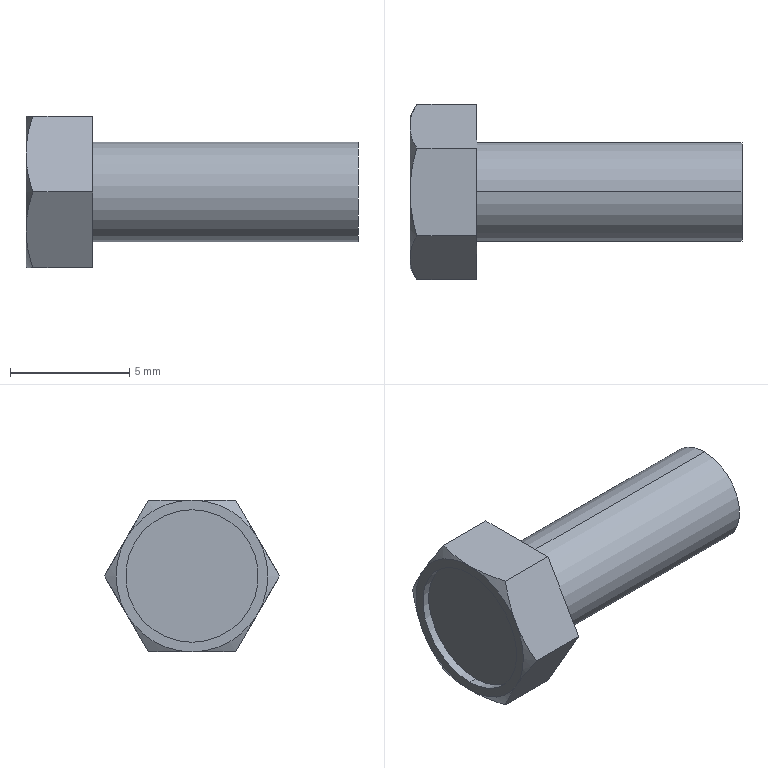Part | SolidWorks | features BaseBody 1 | 1 solid | 20 faces | box 13.907 x 7.332 x 6.35 mm | volume 240.264 mm3 | plane 10 | cone 6 | cylinder 4 | commonest cylinder face diameters 4.166 x2 5.556 x2
STEP:
#1=CARTESIAN_POINT('',(0.3493,0.,2.778));
#2=VERTEX_POINT('',#1);
#3=CARTESIAN_POINT('',(0.3493,0.,-2.778));
#4=VERTEX_POINT('',#3);
#5=CARTESIAN_POINT('',(0.3493,0.,0.));
#6=DIRECTION('',(1.,0.,0.));
#7=DIRECTION('',(0.,0.,1.));
#8=AXIS2_PLACEMENT_3D('',#5,#6,#7);
#9=CIRCLE('',#8,2.778);
#10=EDGE_CURVE('',#2,#4,#9,.T.);
#11=ORIENTED_EDGE('',*,*,#10,.T.);
#12=CARTESIAN_POINT('',(0.,0.,-2.778));
#13=VERTEX_POINT('',#12);
#14=CARTESIAN_POINT('',(0.3493,0.,-2.778));
#15=DIRECTION('',(-1.,0.,0.));
#16=VECTOR('',#15,1000.);
#17=LINE('',#14,#16);
#18=EDGE_CURVE('',#4,#13,#17,.T.);
#19=ORIENTED_EDGE('',*,*,#18,.T.);
#20=CARTESIAN_POINT('',(0.,0.,2.778));
#21=VERTEX_POINT('',#20);
#22=CARTESIAN_POINT('',(0.,0.,0.));
#23=DIRECTION('',(-1.,0.,0.));
#24=DIRECTION('',(0.,0.,1.));
#25=AXIS2_PLACEMENT_3D('',#22,#23,#24);
#26=CIRCLE('',#25,2.778);
#27=EDGE_CURVE('',#13,#21,#26,.T.);
#28=ORIENTED_EDGE('',*,*,#27,.T.);
#29=CARTESIAN_POINT('',(0.3493,0.,2.778));
#30=DIRECTION('',(-1.,0.,0.));
#31=VECTOR('',#30,1000.);
#32=LINE('',#29,#31);
#33=EDGE_CURVE('',#2,#21,#32,.T.);
#34=ORIENTED_EDGE('',*,*,#33,.F.);
#35=EDGE_LOOP('',(#11,#19,#28,#34));
#36=FACE_OUTER_BOUND('',#35,.T.);
#37=CARTESIAN_POINT('',(0.3493,0.,0.));
#38=DIRECTION('',(-1.,0.,0.));
#39=DIRECTION('',(0.,0.,1.));
#40=AXIS2_PLACEMENT_3D('',#37,#38,#39);
#41=CYLINDRICAL_SURFACE('',#40,2.778);
#42=ADVANCED_FACE('',(#36),#41,.F.);
#43=CARTESIAN_POINT('',(13.907,0.,-2.083));
#44=VERTEX_POINT('',#43);
#45=CARTESIAN_POINT('',(13.907,0.,2.083));
#46=VERTEX_POINT('',#45);
#47=CARTESIAN_POINT('',(13.907,0.,0.));
#48=DIRECTION('',(1.,0.,0.));
#49=DIRECTION('',(0.,0.,1.));
#50=AXIS2_PLACEMENT_3D('',#47,#48,#49);
#51=CIRCLE('',#50,2.083);
#52=EDGE_CURVE('',#44,#46,#51,.T.);
#53=ORIENTED_EDGE('',*,*,#52,.F.);
#54=CARTESIAN_POINT('',(2.794,0.,-2.083));
#55=VERTEX_POINT('',#54);
#56=CARTESIAN_POINT('',(13.907,0.,-2.083));
#57=DIRECTION('',(-1.,0.,0.));
#58=VECTOR('',#57,1000.);
#59=LINE('',#56,#58);
#60=EDGE_CURVE('',#44,#55,#59,.T.);
#61=ORIENTED_EDGE('',*,*,#60,.T.);
#62=CARTESIAN_POINT('',(2.794,0.,2.083));
#63=VERTEX_POINT('',#62);
#64=CARTESIAN_POINT('',(2.794,0.,0.));
#65=DIRECTION('',(1.,0.,0.));
#66=DIRECTION('',(0.,0.,1.));
#67=AXIS2_PLACEMENT_3D('',#64,#65,#66);
#68=CIRCLE('',#67,2.083);
#69=EDGE_CURVE('',#55,#63,#68,.T.);
#70=ORIENTED_EDGE('',*,*,#69,.T.);
#71=CARTESIAN_POINT('',(13.907,0.,2.083));
#72=DIRECTION('',(-1.,0.,0.));
#73=VECTOR('',#72,1000.);
#74=LINE('',#71,#73);
#75=EDGE_CURVE('',#46,#63,#74,.T.);
#76=ORIENTED_EDGE('',*,*,#75,.F.);
#77=EDGE_LOOP('',(#53,#61,#70,#76));
#78=FACE_OUTER_BOUND('',#77,.T.);
#79=CARTESIAN_POINT('',(13.907,0.,0.));
#80=DIRECTION('',(-1.,0.,0.));
#81=DIRECTION('',(0.,0.,1.));
#82=AXIS2_PLACEMENT_3D('',#79,#80,#81);
#83=CYLINDRICAL_SURFACE('',#82,2.083);
#84=ADVANCED_FACE('',(#78),#83,.T.);
#85=ORIENTED_EDGE('',*,*,#18,.F.);
#86=CARTESIAN_POINT('',(0.3493,0.,0.));
#87=DIRECTION('',(1.,0.,0.));
#88=DIRECTION('',(0.,0.,1.));
#89=AXIS2_PLACEMENT_3D('',#86,#87,#88);
#90=CIRCLE('',#89,2.778);
#91=EDGE_CURVE('',#4,#2,#90,.T.);
#92=ORIENTED_EDGE('',*,*,#91,.T.);
#93=ORIENTED_EDGE('',*,*,#33,.T.);
#94=CARTESIAN_POINT('',(0.,0.,0.));
#95=DIRECTION('',(-1.,0.,0.));
#96=DIRECTION('',(0.,0.,1.));
#97=AXIS2_PLACEMENT_3D('',#94,#95,#96);
#98=CIRCLE('',#97,2.778);
#99=EDGE_CURVE('',#21,#13,#98,.T.);
#100=ORIENTED_EDGE('',*,*,#99,.T.);
#101=EDGE_LOOP('',(#85,#92,#93,#100));
#102=FACE_OUTER_BOUND('',#101,.T.);
#103=CARTESIAN_POINT('',(0.3493,0.,0.));
#104=DIRECTION('',(-1.,0.,0.));
#105=DIRECTION('',(0.,0.,1.));
#106=AXIS2_PLACEMENT_3D('',#103,#104,#105);
#107=CYLINDRICAL_SURFACE('',#106,2.778);
#108=ADVANCED_FACE('',(#102),#107,.F.);
#109=ORIENTED_EDGE('',*,*,#99,.F.);
#110=ORIENTED_EDGE('',*,*,#27,.F.);
#111=EDGE_LOOP('',(#109,#110));
#112=FACE_BOUND('',#111,.T.);
#113=CARTESIAN_POINT('',(0.000000003,-2.75,-1.588));
#114=VERTEX_POINT('',#113);
#115=CARTESIAN_POINT('',(0.000000006,-2.75,1.588));
#116=VERTEX_POINT('',#115);
#117=CARTESIAN_POINT('',(0.000000006,0.,0.));
#118=DIRECTION('',(-1.,0.,0.));
#119=DIRECTION('',(0.,0.,-1.));
#120=AXIS2_PLACEMENT_3D('',#117,#118,#119);
#121=CIRCLE('',#120,3.175);
#122=EDGE_CURVE('',#114,#116,#121,.T.);
#123=ORIENTED_EDGE('',*,*,#122,.T.);
#124=CARTESIAN_POINT('',(0.,-0.000000001,3.175));
#125=VERTEX_POINT('',#124);
#126=CARTESIAN_POINT('',(0.,0.,0.));
#127=DIRECTION('',(-1.,0.,0.));
#128=DIRECTION('',(0.,0.,-1.));
#129=AXIS2_PLACEMENT_3D('',#126,#127,#128);
#130=CIRCLE('',#129,3.175);
#131=EDGE_CURVE('',#116,#125,#130,.T.);
#132=ORIENTED_EDGE('',*,*,#131,.T.);
#133=CARTESIAN_POINT('',(0.000000003,2.75,1.588));
#134=VERTEX_POINT('',#133);
#135=CARTESIAN_POINT('',(0.,0.,0.));
#136=DIRECTION('',(-1.,0.,0.));
#137=DIRECTION('',(0.,0.,-1.));
#138=AXIS2_PLACEMENT_3D('',#135,#136,#137);
#139=CIRCLE('',#138,3.175);
#140=EDGE_CURVE('',#125,#134,#139,.T.);
#141=ORIENTED_EDGE('',*,*,#140,.T.);
#142=CARTESIAN_POINT('',(0.000000006,2.75,-1.588));
#143=VERTEX_POINT('',#142);
#144=CARTESIAN_POINT('',(0.000000006,0.,0.));
#145=DIRECTION('',(-1.,0.,0.));
#146=DIRECTION('',(0.,0.,-1.));
#147=AXIS2_PLACEMENT_3D('',#144,#145,#146);
#148=CIRCLE('',#147,3.175);
#149=EDGE_CURVE('',#134,#143,#148,.T.);
#150=ORIENTED_EDGE('',*,*,#149,.T.);
#151=CARTESIAN_POINT('',(0.000000003,0.,-3.175));
#152=VERTEX_POINT('',#151);
#153=CARTESIAN_POINT('',(0.000000006,0.,0.));
#154=DIRECTION('',(-1.,0.,0.));
#155=DIRECTION('',(0.,0.,-1.));
#156=AXIS2_PLACEMENT_3D('',#153,#154,#155);
#157=CIRCLE('',#156,3.175);
#158=EDGE_CURVE('',#143,#152,#157,.T.);
#159=ORIENTED_EDGE('',*,*,#158,.T.);
#160=CARTESIAN_POINT('',(0.,0.,0.));
#161=DIRECTION('',(-1.,0.,0.));
#162=DIRECTION('',(0.,0.,-1.));
#163=AXIS2_PLACEMENT_3D('',#160,#161,#162);
#164=CIRCLE('',#163,3.175);
#165=EDGE_CURVE('',#152,#114,#164,.T.);
#166=ORIENTED_EDGE('',*,*,#165,.T.);
#167=EDGE_LOOP('',(#123,#132,#141,#150,#159,#166));
#168=FACE_OUTER_BOUND('',#167,.T.);
#169=CARTESIAN_POINT('',(0.,-3.213,-3.213));
#170=DIRECTION('',(-1.,0.,0.));
#171=DIRECTION('',(0.,0.,1.));
#172=AXIS2_PLACEMENT_3D('',#169,#170,#171);
#173=PLANE('',#172);
#174=ADVANCED_FACE('',(#112,#168),#173,.T.);
#175=ORIENTED_EDGE('',*,*,#10,.F.);
#176=ORIENTED_EDGE('',*,*,#91,.F.);
#177=EDGE_LOOP('',(#175,#176));
#178=FACE_OUTER_BOUND('',#177,.T.);
#179=CARTESIAN_POINT('',(0.3493,-2.811,2.811));
#180=DIRECTION('',(1.,0.,0.));
#181=DIRECTION('',(0.,0.,-1.));
#182=AXIS2_PLACEMENT_3D('',#179,#180,#181);
#183=PLANE('',#182);
#184=ADVANCED_FACE('',(#178),#183,.F.);
#185=CARTESIAN_POINT('',(0.2836,-1.833,3.175));
#186=VERTEX_POINT('',#185);
#187=CARTESIAN_POINT('',(0.2836,-1.833,3.175));
#188=CARTESIAN_POINT('',(0.1107,-2.133,2.656));
#189=CARTESIAN_POINT('',(0.000000006,-2.437,2.129));
#190=CARTESIAN_POINT('',(0.000000006,-2.75,1.588));
#191=B_SPLINE_CURVE_WITH_KNOTS('',3,(#187,#188,#189,#190),.UNSPECIFIED.,.F.,.F.,(4,4),(0.,0.001855),.UNSPECIFIED.);
#192=EDGE_CURVE('',#186,#116,#191,.T.);
#193=ORIENTED_EDGE('',*,*,#192,.F.);
#194=CARTESIAN_POINT('',(0.,-0.000000001,3.175));
#195=CARTESIAN_POINT('',(0.,-0.6257,3.175));
#196=CARTESIAN_POINT('',(0.1107,-1.234,3.175));
#197=CARTESIAN_POINT('',(0.2836,-1.833,3.175));
#198=B_SPLINE_CURVE_WITH_KNOTS('',3,(#194,#195,#196,#197),.UNSPECIFIED.,.F.,.F.,(4,4),(0.,0.001855),.UNSPECIFIED.);
#199=EDGE_CURVE('',#125,#186,#198,.T.);
#200=ORIENTED_EDGE('',*,*,#199,.F.);
#201=ORIENTED_EDGE('',*,*,#131,.F.);
#202=EDGE_LOOP('',(#193,#200,#201));
#203=FACE_OUTER_BOUND('',#202,.T.);
#204=CARTESIAN_POINT('',(0.,0.,0.));
#205=DIRECTION('',(1.,0.,0.));
#206=DIRECTION('',(0.,0.,-1.));
#207=AXIS2_PLACEMENT_3D('',#204,#205,#206);
#208=CONICAL_SURFACE('',#207,3.175,1.047);
#209=ADVANCED_FACE('',(#203),#208,.T.);
#210=CARTESIAN_POINT('',(0.2836,-3.666,0.));
#211=VERTEX_POINT('',#210);
#212=CARTESIAN_POINT('',(0.2836,-3.666,0.));
#213=CARTESIAN_POINT('',(0.1107,-3.367,-0.5187));
#214=CARTESIAN_POINT('',(0.000000006,-3.062,-1.046));
#215=CARTESIAN_POINT('',(0.000000003,-2.75,-1.588));
#216=B_SPLINE_CURVE_WITH_KNOTS('',3,(#212,#213,#214,#215),.UNSPECIFIED.,.F.,.F.,(4,4),(0.,0.001855),.UNSPECIFIED.);
#217=EDGE_CURVE('',#211,#114,#216,.T.);
#218=ORIENTED_EDGE('',*,*,#217,.F.);
#219=CARTESIAN_POINT('',(0.000000006,-2.75,1.588));
#220=CARTESIAN_POINT('',(0.000000006,-3.062,1.046));
#221=CARTESIAN_POINT('',(0.1107,-3.367,0.5187));
#222=CARTESIAN_POINT('',(0.2836,-3.666,0.));
#223=B_SPLINE_CURVE_WITH_KNOTS('',3,(#219,#220,#221,#222),.UNSPECIFIED.,.F.,.F.,(4,4),(0.,0.001855),.UNSPECIFIED.);
#224=EDGE_CURVE('',#116,#211,#223,.T.);
#225=ORIENTED_EDGE('',*,*,#224,.F.);
#226=ORIENTED_EDGE('',*,*,#122,.F.);
#227=EDGE_LOOP('',(#218,#225,#226));
#228=FACE_OUTER_BOUND('',#227,.T.);
#229=CARTESIAN_POINT('',(0.000000006,0.,0.));
#230=DIRECTION('',(1.,0.,0.));
#231=DIRECTION('',(0.,0.,-1.));
#232=AXIS2_PLACEMENT_3D('',#229,#230,#231);
#233=CONICAL_SURFACE('',#232,3.175,1.047);
#234=ADVANCED_FACE('',(#228),#233,.T.);
#235=CARTESIAN_POINT('',(0.2836,-1.833,-3.175));
#236=VERTEX_POINT('',#235);
#237=CARTESIAN_POINT('',(0.000000003,-2.75,-1.588));
#238=CARTESIAN_POINT('',(0.000000006,-2.437,-2.129));
#239=CARTESIAN_POINT('',(0.1107,-2.133,-2.656));
#240=CARTESIAN_POINT('',(0.2836,-1.833,-3.175));
#241=B_SPLINE_CURVE_WITH_KNOTS('',3,(#237,#238,#239,#240),.UNSPECIFIED.,.F.,.F.,(4,4),(0.,0.001855),.UNSPECIFIED.);
#242=EDGE_CURVE('',#114,#236,#241,.T.);
#243=ORIENTED_EDGE('',*,*,#242,.F.);
#244=ORIENTED_EDGE('',*,*,#165,.F.);
#245=CARTESIAN_POINT('',(0.2836,-1.833,-3.175));
#246=CARTESIAN_POINT('',(0.1107,-1.234,-3.175));
#247=CARTESIAN_POINT('',(0.,-0.6257,-3.175));
#248=CARTESIAN_POINT('',(0.000000003,0.,-3.175));
#249=B_SPLINE_CURVE_WITH_KNOTS('',3,(#245,#246,#247,#248),.UNSPECIFIED.,.F.,.F.,(4,4),(0.,0.001855),.UNSPECIFIED.);
#250=EDGE_CURVE('',#236,#152,#249,.T.);
#251=ORIENTED_EDGE('',*,*,#250,.F.);
#252=EDGE_LOOP('',(#243,#244,#251));
#253=FACE_OUTER_BOUND('',#252,.T.);
#254=CARTESIAN_POINT('',(0.,0.,0.));
#255=DIRECTION('',(1.,0.,0.));
#256=DIRECTION('',(0.,0.,-1.));
#257=AXIS2_PLACEMENT_3D('',#254,#255,#256);
#258=CONICAL_SURFACE('',#257,3.175,1.047);
#259=ADVANCED_FACE('',(#253),#258,.T.);
#260=CARTESIAN_POINT('',(0.2836,1.833,-3.175));
#261=VERTEX_POINT('',#260);
#262=CARTESIAN_POINT('',(0.000000003,0.,-3.175));
#263=CARTESIAN_POINT('',(0.,0.6257,-3.175));
#264=CARTESIAN_POINT('',(0.1107,1.234,-3.175));
#265=CARTESIAN_POINT('',(0.2836,1.833,-3.175));
#266=B_SPLINE_CURVE_WITH_KNOTS('',3,(#262,#263,#264,#265),.UNSPECIFIED.,.F.,.F.,(4,4),(0.,0.001855),.UNSPECIFIED.);
#267=EDGE_CURVE('',#152,#261,#266,.T.);
#268=ORIENTED_EDGE('',*,*,#267,.F.);
#269=ORIENTED_EDGE('',*,*,#158,.F.);
#270=CARTESIAN_POINT('',(0.2836,1.833,-3.175));
#271=CARTESIAN_POINT('',(0.1107,2.133,-2.656));
#272=CARTESIAN_POINT('',(0.000000006,2.437,-2.129));
#273=CARTESIAN_POINT('',(0.000000006,2.75,-1.588));
#274=B_SPLINE_CURVE_WITH_KNOTS('',3,(#270,#271,#272,#273),.UNSPECIFIED.,.F.,.F.,(4,4),(0.,0.001855),.UNSPECIFIED.);
#275=EDGE_CURVE('',#261,#143,#274,.T.);
#276=ORIENTED_EDGE('',*,*,#275,.F.);
#277=EDGE_LOOP('',(#268,#269,#276));
#278=FACE_OUTER_BOUND('',#277,.T.);
#279=CARTESIAN_POINT('',(0.,0.,0.));
#280=DIRECTION('',(1.,0.,0.));
#281=DIRECTION('',(0.,0.,-1.));
#282=AXIS2_PLACEMENT_3D('',#279,#280,#281);
#283=CONICAL_SURFACE('',#282,3.175,1.047);
#284=ADVANCED_FACE('',(#278),#283,.T.);
#285=CARTESIAN_POINT('',(0.2836,3.666,0.));
#286=VERTEX_POINT('',#285);
#287=CARTESIAN_POINT('',(0.000000006,2.75,-1.588));
#288=CARTESIAN_POINT('',(0.000000006,3.062,-1.046));
#289=CARTESIAN_POINT('',(0.1107,3.367,-0.5187));
#290=CARTESIAN_POINT('',(0.2836,3.666,0.));
#291=B_SPLINE_CURVE_WITH_KNOTS('',3,(#287,#288,#289,#290),.UNSPECIFIED.,.F.,.F.,(4,4),(0.,0.001855),.UNSPECIFIED.);
#292=EDGE_CURVE('',#143,#286,#291,.T.);
#293=ORIENTED_EDGE('',*,*,#292,.F.);
#294=ORIENTED_EDGE('',*,*,#149,.F.);
#295=CARTESIAN_POINT('',(0.2836,3.666,0.));
#296=CARTESIAN_POINT('',(0.1107,3.367,0.5187));
#297=CARTESIAN_POINT('',(0.000000006,3.062,1.046));
#298=CARTESIAN_POINT('',(0.000000003,2.75,1.588));
#299=B_SPLINE_CURVE_WITH_KNOTS('',3,(#295,#296,#297,#298),.UNSPECIFIED.,.F.,.F.,(4,4),(0.,0.001855),.UNSPECIFIED.);
#300=EDGE_CURVE('',#286,#134,#299,.T.);
#301=ORIENTED_EDGE('',*,*,#300,.F.);
#302=EDGE_LOOP('',(#293,#294,#301));
#303=FACE_OUTER_BOUND('',#302,.T.);
#304=CARTESIAN_POINT('',(0.000000006,0.,0.));
#305=DIRECTION('',(1.,0.,0.));
#306=DIRECTION('',(0.,0.,-1.));
#307=AXIS2_PLACEMENT_3D('',#304,#305,#306);
#308=CONICAL_SURFACE('',#307,3.175,1.047);
#309=ADVANCED_FACE('',(#303),#308,.T.);
#310=CARTESIAN_POINT('',(0.2836,1.833,3.175));
#311=VERTEX_POINT('',#310);
#312=CARTESIAN_POINT('',(0.2836,1.833,3.175));
#313=CARTESIAN_POINT('',(0.1107,1.234,3.175));
#314=CARTESIAN_POINT('',(0.,0.6257,3.175));
#315=CARTESIAN_POINT('',(0.,-0.000000001,3.175));
#316=B_SPLINE_CURVE_WITH_KNOTS('',3,(#312,#313,#314,#315),.UNSPECIFIED.,.F.,.F.,(4,4),(0.,0.001855),.UNSPECIFIED.);
#317=EDGE_CURVE('',#311,#125,#316,.T.);
#318=ORIENTED_EDGE('',*,*,#317,.F.);
#319=CARTESIAN_POINT('',(0.000000003,2.75,1.588));
#320=CARTESIAN_POINT('',(0.000000006,2.437,2.129));
#321=CARTESIAN_POINT('',(0.1107,2.133,2.656));
#322=CARTESIAN_POINT('',(0.2836,1.833,3.175));
#323=B_SPLINE_CURVE_WITH_KNOTS('',3,(#319,#320,#321,#322),.UNSPECIFIED.,.F.,.F.,(4,4),(0.,0.001855),.UNSPECIFIED.);
#324=EDGE_CURVE('',#134,#311,#323,.T.);
#325=ORIENTED_EDGE('',*,*,#324,.F.);
#326=ORIENTED_EDGE('',*,*,#140,.F.);
#327=EDGE_LOOP('',(#318,#325,#326));
#328=FACE_OUTER_BOUND('',#327,.T.);
#329=CARTESIAN_POINT('',(0.,0.,0.));
#330=DIRECTION('',(1.,0.,0.));
#331=DIRECTION('',(0.,0.,-1.));
#332=AXIS2_PLACEMENT_3D('',#329,#330,#331);
#333=CONICAL_SURFACE('',#332,3.175,1.047);
#334=ADVANCED_FACE('',(#328),#333,.T.);
#335=ORIENTED_EDGE('',*,*,#192,.T.);
#336=ORIENTED_EDGE('',*,*,#224,.T.);
#337=CARTESIAN_POINT('',(2.794,-3.666,0.));
#338=VERTEX_POINT('',#337);
#339=CARTESIAN_POINT('',(1.389,-3.666,0.));
#340=DIRECTION('',(1.,0.,0.));
#341=VECTOR('',#340,1000.);
#342=LINE('',#339,#341);
#343=EDGE_CURVE('',#211,#338,#342,.T.);
#344=ORIENTED_EDGE('',*,*,#343,.T.);
#345=CARTESIAN_POINT('',(2.794,-1.833,3.175));
#346=VERTEX_POINT('',#345);
#347=CARTESIAN_POINT('',(2.794,-2.75,1.587));
#348=DIRECTION('',(0.,0.5,0.866));
#349=VECTOR('',#348,1000.);
#350=LINE('',#347,#349);
#351=EDGE_CURVE('',#338,#346,#350,.T.);
#352=ORIENTED_EDGE('',*,*,#351,.T.);
#353=CARTESIAN_POINT('',(1.389,-1.833,3.175));
#354=DIRECTION('',(-1.,0.,0.));
#355=VECTOR('',#354,1000.);
#356=LINE('',#353,#355);
#357=EDGE_CURVE('',#346,#186,#356,.T.);
#358=ORIENTED_EDGE('',*,*,#357,.T.);
#359=EDGE_LOOP('',(#335,#336,#344,#352,#358));
#360=FACE_OUTER_BOUND('',#359,.T.);
#361=CARTESIAN_POINT('',(-0.01676,-1.833,3.175));
#362=DIRECTION('',(0.,-0.866,0.5));
#363=DIRECTION('',(0.,-0.5,-0.866));
#364=AXIS2_PLACEMENT_3D('',#361,#362,#363);
#365=PLANE('',#364);
#366=ADVANCED_FACE('',(#360),#365,.T.);
#367=ORIENTED_EDGE('',*,*,#317,.T.);
#368=ORIENTED_EDGE('',*,*,#199,.T.);
#369=ORIENTED_EDGE('',*,*,#357,.F.);
#370=CARTESIAN_POINT('',(2.794,1.833,3.175));
#371=VERTEX_POINT('',#370);
#372=CARTESIAN_POINT('',(2.794,0.,3.175));
#373=DIRECTION('',(0.,1.,0.));
#374=VECTOR('',#373,1000.);
#375=LINE('',#372,#374);
#376=EDGE_CURVE('',#346,#371,#375,.T.);
#377=ORIENTED_EDGE('',*,*,#376,.T.);
#378=CARTESIAN_POINT('',(1.389,1.833,3.175));
#379=DIRECTION('',(-1.,0.,0.));
#380=VECTOR('',#379,1000.);
#381=LINE('',#378,#380);
#382=EDGE_CURVE('',#371,#311,#381,.T.);
#383=ORIENTED_EDGE('',*,*,#382,.T.);
#384=EDGE_LOOP('',(#367,#368,#369,#377,#383));
#385=FACE_OUTER_BOUND('',#384,.T.);
#386=CARTESIAN_POINT('',(-0.01676,1.833,3.175));
#387=DIRECTION('',(0.,0.,1.));
#388=DIRECTION('',(0.,-1.,0.));
#389=AXIS2_PLACEMENT_3D('',#386,#387,#388);
#390=PLANE('',#389);
#391=ADVANCED_FACE('',(#385),#390,.T.);
#392=ORIENTED_EDGE('',*,*,#217,.T.);
#393=ORIENTED_EDGE('',*,*,#242,.T.);
#394=CARTESIAN_POINT('',(2.794,-1.833,-3.175));
#395=VERTEX_POINT('',#394);
#396=CARTESIAN_POINT('',(1.389,-1.833,-3.175));
#397=DIRECTION('',(1.,0.,0.));
#398=VECTOR('',#397,1000.);
#399=LINE('',#396,#398);
#400=EDGE_CURVE('',#236,#395,#399,.T.);
#401=ORIENTED_EDGE('',*,*,#400,.T.);
#402=CARTESIAN_POINT('',(2.794,-2.75,-1.587));
#403=DIRECTION('',(0.,-0.5,0.866));
#404=VECTOR('',#403,1000.);
#405=LINE('',#402,#404);
#406=EDGE_CURVE('',#395,#338,#405,.T.);
#407=ORIENTED_EDGE('',*,*,#406,.T.);
#408=ORIENTED_EDGE('',*,*,#343,.F.);
#409=EDGE_LOOP('',(#392,#393,#401,#407,#408));
#410=FACE_OUTER_BOUND('',#409,.T.);
#411=CARTESIAN_POINT('',(-0.01676,-3.666,0.));
#412=DIRECTION('',(0.,-0.866,-0.5));
#413=DIRECTION('',(0.,0.5,-0.866));
#414=AXIS2_PLACEMENT_3D('',#411,#412,#413);
#415=PLANE('',#414);
#416=ADVANCED_FACE('',(#410),#415,.T.);
#417=ORIENTED_EDGE('',*,*,#250,.T.);
#418=ORIENTED_EDGE('',*,*,#267,.T.);
#419=CARTESIAN_POINT('',(2.794,1.833,-3.175));
#420=VERTEX_POINT('',#419);
#421=CARTESIAN_POINT('',(1.389,1.833,-3.175));
#422=DIRECTION('',(1.,0.,0.));
#423=VECTOR('',#422,1000.);
#424=LINE('',#421,#423);
#425=EDGE_CURVE('',#261,#420,#424,.T.);
#426=ORIENTED_EDGE('',*,*,#425,.T.);
#427=CARTESIAN_POINT('',(2.794,0.,-3.175));
#428=DIRECTION('',(0.,-1.,0.));
#429=VECTOR('',#428,1000.);
#430=LINE('',#427,#429);
#431=EDGE_CURVE('',#420,#395,#430,.T.);
#432=ORIENTED_EDGE('',*,*,#431,.T.);
#433=ORIENTED_EDGE('',*,*,#400,.F.);
#434=EDGE_LOOP('',(#417,#418,#426,#432,#433));
#435=FACE_OUTER_BOUND('',#434,.T.);
#436=CARTESIAN_POINT('',(-0.01676,-1.833,-3.175));
#437=DIRECTION('',(0.,0.,-1.));
#438=DIRECTION('',(0.,1.,0.));
#439=AXIS2_PLACEMENT_3D('',#436,#437,#438);
#440=PLANE('',#439);
#441=ADVANCED_FACE('',(#435),#440,.T.);
#442=ORIENTED_EDGE('',*,*,#275,.T.);
#443=ORIENTED_EDGE('',*,*,#292,.T.);
#444=CARTESIAN_POINT('',(2.794,3.666,0.));
#445=VERTEX_POINT('',#444);
#446=CARTESIAN_POINT('',(1.389,3.666,0.));
#447=DIRECTION('',(1.,0.,0.));
#448=VECTOR('',#447,1000.);
#449=LINE('',#446,#448);
#450=EDGE_CURVE('',#286,#445,#449,.T.);
#451=ORIENTED_EDGE('',*,*,#450,.T.);
#452=CARTESIAN_POINT('',(2.794,2.75,-1.587));
#453=DIRECTION('',(0.,-0.5,-0.866));
#454=VECTOR('',#453,1000.);
#455=LINE('',#452,#454);
#456=EDGE_CURVE('',#445,#420,#455,.T.);
#457=ORIENTED_EDGE('',*,*,#456,.T.);
#458=ORIENTED_EDGE('',*,*,#425,.F.);
#459=EDGE_LOOP('',(#442,#443,#451,#457,#458));
#460=FACE_OUTER_BOUND('',#459,.T.);
#461=CARTESIAN_POINT('',(-0.01676,1.833,-3.175));
#462=DIRECTION('',(0.,0.866,-0.5));
#463=DIRECTION('',(0.,0.5,0.866));
#464=AXIS2_PLACEMENT_3D('',#461,#462,#463);
#465=PLANE('',#464);
#466=ADVANCED_FACE('',(#460),#465,.T.);
#467=ORIENTED_EDGE('',*,*,#300,.T.);
#468=ORIENTED_EDGE('',*,*,#324,.T.);
#469=ORIENTED_EDGE('',*,*,#382,.F.);
#470=CARTESIAN_POINT('',(2.794,2.75,1.587));
#471=DIRECTION('',(0.,0.5,-0.866));
#472=VECTOR('',#471,1000.);
#473=LINE('',#470,#472);
#474=EDGE_CURVE('',#371,#445,#473,.T.);
#475=ORIENTED_EDGE('',*,*,#474,.T.);
#476=ORIENTED_EDGE('',*,*,#450,.F.);
#477=EDGE_LOOP('',(#467,#468,#469,#475,#476));
#478=FACE_OUTER_BOUND('',#477,.T.);
#479=CARTESIAN_POINT('',(-0.01676,3.666,0.));
#480=DIRECTION('',(0.,0.866,0.5));
#481=DIRECTION('',(0.,-0.5,0.866));
#482=AXIS2_PLACEMENT_3D('',#479,#480,#481);
#483=PLANE('',#482);
#484=ADVANCED_FACE('',(#478),#483,.T.);
#485=CARTESIAN_POINT('',(2.794,0.,0.));
#486=DIRECTION('',(1.,0.,0.));
#487=DIRECTION('',(0.,0.,1.));
#488=AXIS2_PLACEMENT_3D('',#485,#486,#487);
#489=CIRCLE('',#488,2.083);
#490=EDGE_CURVE('',#63,#55,#489,.T.);
#491=ORIENTED_EDGE('',*,*,#490,.F.);
#492=ORIENTED_EDGE('',*,*,#69,.F.);
#493=EDGE_LOOP('',(#491,#492));
#494=FACE_BOUND('',#493,.T.);
#495=ORIENTED_EDGE('',*,*,#351,.F.);
#496=ORIENTED_EDGE('',*,*,#406,.F.);
#497=ORIENTED_EDGE('',*,*,#431,.F.);
#498=ORIENTED_EDGE('',*,*,#456,.F.);
#499=ORIENTED_EDGE('',*,*,#474,.F.);
#500=ORIENTED_EDGE('',*,*,#376,.F.);
#501=EDGE_LOOP('',(#495,#496,#497,#498,#499,#500));
#502=FACE_OUTER_BOUND('',#501,.T.);
#503=CARTESIAN_POINT('',(2.794,-3.71,-3.175));
#504=DIRECTION('',(-1.,0.,0.));
#505=DIRECTION('',(0.,0.,1.));
#506=AXIS2_PLACEMENT_3D('',#503,#504,#505);
#507=PLANE('',#506);
#508=ADVANCED_FACE('',(#494,#502),#507,.F.);
#509=ORIENTED_EDGE('',*,*,#60,.F.);
#510=CARTESIAN_POINT('',(13.907,0.,0.));
#511=DIRECTION('',(1.,0.,0.));
#512=DIRECTION('',(0.,0.,1.));
#513=AXIS2_PLACEMENT_3D('',#510,#511,#512);
#514=CIRCLE('',#513,2.083);
#515=EDGE_CURVE('',#46,#44,#514,.T.);
#516=ORIENTED_EDGE('',*,*,#515,.F.);
#517=ORIENTED_EDGE('',*,*,#75,.T.);
#518=ORIENTED_EDGE('',*,*,#490,.T.);
#519=EDGE_LOOP('',(#509,#516,#517,#518));
#520=FACE_OUTER_BOUND('',#519,.T.);
#521=CARTESIAN_POINT('',(13.907,0.,0.));
#522=DIRECTION('',(-1.,0.,0.));
#523=DIRECTION('',(0.,0.,1.));
#524=AXIS2_PLACEMENT_3D('',#521,#522,#523);
#525=CYLINDRICAL_SURFACE('',#524,2.083);
#526=ADVANCED_FACE('',(#520),#525,.T.);
#527=ORIENTED_EDGE('',*,*,#515,.T.);
#528=ORIENTED_EDGE('',*,*,#52,.T.);
#529=EDGE_LOOP('',(#527,#528));
#530=FACE_OUTER_BOUND('',#529,.T.);
#531=CARTESIAN_POINT('',(13.907,-2.108,2.108));
#532=DIRECTION('',(1.,0.,0.));
#533=DIRECTION('',(0.,0.,-1.));
#534=AXIS2_PLACEMENT_3D('',#531,#532,#533);
#535=PLANE('',#534);
#536=ADVANCED_FACE('',(#530),#535,.T.);
#537=CLOSED_SHELL('',(#42,#84,#108,#174,#184,#209,#234,#259,#284,#309,#334,#366,#391,#416,#441,#466,#484,#508,#526,#536));
#538=MANIFOLD_SOLID_BREP('',#537);
#539=CARTESIAN_POINT('',(0.,0.,0.));
#540=DIRECTION('',(0.,0.,1.));
#541=DIRECTION('',(1.,0.,0.));
#542=AXIS2_PLACEMENT_3D('',#539,#540,#541);
#543=(LENGTH_UNIT()NAMED_UNIT(*)SI_UNIT(.MILLI.,.METRE.));
#544=UNCERTAINTY_MEASURE_WITH_UNIT(LENGTH_MEASURE(0.00001),#543,'','');
#545=(NAMED_UNIT(*)PLANE_ANGLE_UNIT()SI_UNIT($,.RADIAN.));
#546=(NAMED_UNIT(*)SI_UNIT($,.STERADIAN.)SOLID_ANGLE_UNIT());
#547=(GEOMETRIC_REPRESENTATION_CONTEXT(3)GLOBAL_UNCERTAINTY_ASSIGNED_CONTEXT((#544))GLOBAL_UNIT_ASSIGNED_CONTEXT((#543,#545,#546))REPRESENTATION_CONTEXT('',''));
#548=ADVANCED_BREP_SHAPE_REPRESENTATION('',(#538,#542),#547);